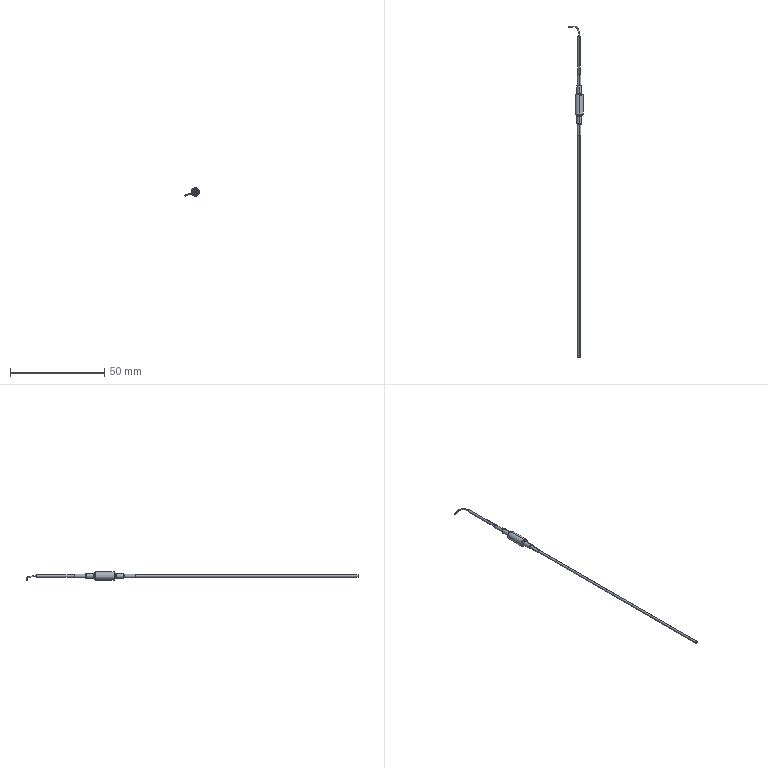Part | SolidWorks | features 3DProfileFeature 2, ICE 2, Revolution 1, Sweep 1 | 1 solid | 47 faces | box 7.759 x 176.005 x 4.43 mm | volume 429.128 mm3 | cylinder 16 | torus 16 | cone 8 | plane 5 | spline 2 | commonest cylinder face diameters 1.3 x4 1.8 x4 2.5 x4 0.5 x2 4.43 x2